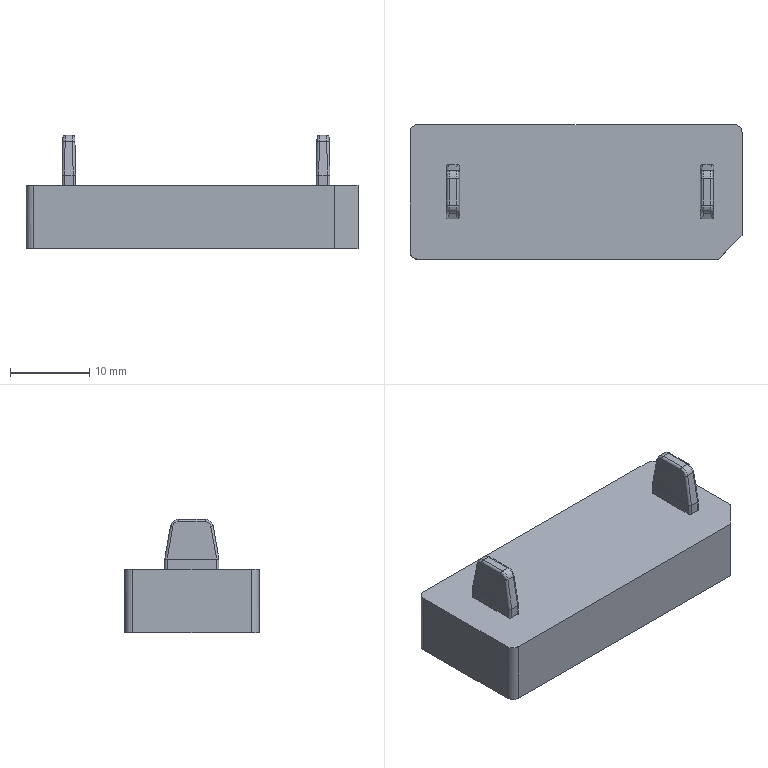NC program | PowerMill | posted by the shop | part box 42 x 17 x 14.346 mm
Lines 3424 to 3987 of 50900:
( TOOL ID   D10_1_1 )
( TOOL DIA. 10. TIP RAD 0 LENGTH 69.52 )
( Z = -.404 )
T3 M6
T4
G91 G28 Z0
G0 G90 G54
M08
S8500 M3
X0 Y0 M8
G43 Z11.796 H3
X-11.962 Y-11.844
Z.796
G1 Z-.404 F360
X-13.457 Y-6.785 F600
X-13.817 Y6.954
X-14.302 Y7.052
X-14.75 Y7.102
X-15.198 Y7.112
X-15.645 Y7.094
X-16.092 Y7.096
X-16.54 Y7.07
X-16.988 Y7.01
X-17.435 Y6.905
X-17.707 Y6.821
X-17.347 Y-6.889
G0 Z3.996
G1 X20.165 Y-11.853 F10000
G0 Z.796
G1 Z-.404 F360
X18.675 Y-6.793 F600
X18.364 Y6.949
X17.881 Y7.048
X17.433 Y7.101
X16.985 Y7.112
X16.538 Y7.091
X16.091 Y7.096
X15.643 Y7.073
X15.195 Y7.015
X14.748 Y6.914
X14.478 Y6.832
X14.788 Y-6.884
G0 Z11.796
X0 Y0
Z9.796
X31.535 Y3.509
Z-5.35
G1 Z-6.55 F360
X26.26 F600
X22.67 Y3.361
X22.675 Y-3.109
X22.665 Y-3.417
X22.639 Y-3.723
X22.59 Y-4.077
X22.516 Y-4.426
X22.42 Y-4.769
G2 X20.666 Y-7.385 I-5.297 J1.655
X19.816 Y-7.966 I-3.572 J4.314
G1 X19.515 Y-8.122
X19.205 Y-8.259
X18.887 Y-8.375
G2 X18.117 Y-8.574 I-1.905 J5.767
G1 X17.764 Y-8.625
X17.409 Y-8.657
X16.722 Y-8.666
X15.751 Y-8.657
X15.396 Y-8.625
X15.043 Y-8.574
X14.685 Y-8.497
X14.273 Y-8.375
G2 X13.295 Y-7.939 I1.765 J5.269
G1 X13.017 Y-7.771
X12.749 Y-7.586
X12.494 Y-7.385
G2 X10.74 Y-4.769 I3.544 J4.271
G1 X10.644 Y-4.426
X10.561 Y-4.008
X10.518 Y-3.698
X10.492 Y-3.385
X10.485 Y-3.109
Y3.148
G2 X10.644 Y4.465 I5.803 J-.031
X10.87 Y5.181 I6.382 J-1.628
G1 X11.001 Y5.486
G2 X11.518 Y6.376 I5.36 J-2.52
G1 X11.749 Y6.675
G2 X13.344 Y8.005 I4.289 J-3.522
G1 X13.645 Y8.161
G2 X14.579 Y8.505 I2.378 J-5.018
X16.036 Y8.704 I1.477 J-5.401
G1 X16.722 Y8.705
X17.409 Y8.696
X17.706 Y8.671
G2 X19.909 Y7.951 I-.58 J-5.501
G1 X20.143 Y7.81
G2 X21.193 Y6.928 I-3.119 J-4.776
G1 X21.425 Y6.658
X21.642 Y6.376
G2 X22.01 Y5.782 I-4.881 J-3.437
G1 X22.159 Y5.486
X22.29 Y5.181
X22.412 Y4.831
G2 X22.67 Y3.361 I-5.38 J-1.702
G1 X26.26 Y3.509
G0 Z2.856
G1 X-31.535 Y.02 F10000
G0 Z-5.35
G1 Z-6.55 F360
X-26.26 F600
X-21.675
Y3.148
X-21.665 Y3.456
X-21.639 Y3.763
X-21.59 Y4.116
X-21.516 Y4.465
G2 X-21.29 Y5.181 I6.452 J-1.651
G1 X-21.162 Y5.481
G2 X-20.821 Y6.109 I5.763 J-2.719
X-20.411 Y6.675 I4.853 J-3.078
G1 X-20.193 Y6.928
G2 X-19.666 Y7.424 I4.215 J-3.942
G1 X-19.411 Y7.625
G2 X-16.179 Y8.702 I3.295 J-4.5
G1 X-15.036 Y8.704
X-14.72 Y8.694
X-14.406 Y8.666
X-14.043 Y8.614
X-13.869 Y8.576
G2 X-13.216 Y8.393 I-1.014 J-4.88
G1 X-12.955 Y8.298
X-12.645 Y8.161
X-12.295 Y7.978
X-12.017 Y7.81
X-11.749 Y7.625
X-11.494 Y7.424
G2 X-10.967 Y6.928 I-3.716 J-4.467
G1 X-10.735 Y6.658
X-10.518 Y6.376
G2 X-9.74 Y4.808 I-4.556 J-3.237
G1 X-9.644 Y4.465
G2 X-9.485 Y3.148 I-5.657 J-1.349
G1 Y.174
X.298 Y.21
X.308 Y-3.307
X.291 Y-3.81
G3 X.454 Y-3.98 I.163 J-.006
G1 X.563
G3 X.725 Y-3.807 I0 J.162
G1 X.461 Y.023
G2 X.507 Y3.684 I22.513 J1.548
G1 X.522 Y3.837
G3 X.406 Y3.97 I-.12 J.011
X.28 Y3.847 I-.005 J-.121
G1 X.298 Y.21
X-4.676 Y.192
X-4.688 Y3.403
G3 X-4.911 Y5.299 I-10.314 J-.251
G1 X-4.952 Y5.491
X-5.182 Y6.32
X-5.415 Y6.967
X-5.79 Y7.862
G2 X-5.067 Y8.955 I.724 J.307
G1 X6.068
G2 X6.791 Y7.863 I0 J-.785
G1 X6.51 Y7.203
G3 X5.413 Y.753 I13.041 J-5.537
G1 X5.714 Y-3.871
G3 X6.094 Y-5.986 I10.404 J.779
G1 X6.227 Y-6.412
X6.369 Y-6.809
X6.527 Y-7.201
X6.811 Y-7.863
G2 X6.092 Y-8.954 I-.719 J-.309
G1 X-5.092 Y-8.955
G2 X-5.803 Y-7.843 I0 J.783
G1 X-5.675 Y-7.566
G3 X-5.169 Y-6.25 I-9.851 J4.544
G1 X-5.141 Y-6.161
G3 X-4.664 Y-2.995 I-10.056 J3.133
G1 X-4.676 Y.192
X-9.485 Y.174
Y-3.109
X-9.495 Y-3.417
X-9.521 Y-3.723
X-9.57 Y-4.077
X-9.644 Y-4.426
G2 X-9.87 Y-5.142 I-6.444 J1.648
X-10.518 Y-6.337 I-5.326 J2.114
X-11.202 Y-7.126 I-4.806 J3.47
X-12.017 Y-7.771 I-4.034 J4.265
X-12.955 Y-8.259 I-3.189 J4.984
X-14.043 Y-8.574 I-2.202 J5.557
G1 X-14.396 Y-8.625
X-14.751 Y-8.657
X-15.036 Y-8.664
X-16.409 Y-8.657
G2 X-17.247 Y-8.546 I.3 J5.522
G1 X-17.475 Y-8.497
X-17.887 Y-8.375
X-18.205 Y-8.259
X-18.515 Y-8.122
X-18.816 Y-7.966
G2 X-21.01 Y-5.743 I2.691 J4.85
X-21.42 Y-4.769 I4.921 J2.643
G1 X-21.516 Y-4.426
X-21.59 Y-4.077
X-21.639 Y-3.723
X-21.665 Y-3.417
X-21.675 Y-3.109
Y.02
X-26.26
G0 Z9.796
X0 Y0
X26.008 Y-14.747
Z-13.25
G1 Z-14.45 F360
G3 X22.473 Y-11.211 I-1.768 J1.768 F600
G1 X21.559 Y-12.125
X21.557 Y-12.127
X21.554 Y-12.129
X21.061 Y-12.554
X21.057 Y-12.557
X21.053 Y-12.56
X20.606 Y-12.861
X20.603 Y-12.862
X20.6 Y-12.864
X20.294 Y-13.033
X20.292 Y-13.034
X20.29 Y-13.035
X20.149 Y-13.103
X20.147 Y-13.104
X20.145 Y-13.105
X19.698 Y-13.288
X19.694 Y-13.289
X19.69 Y-13.29
X19.244 Y-13.425
X19.241 Y-13.426
X19.238 Y-13.427
X18.964 Y-13.488
X18.962
X18.96
X18.787 Y-13.519
X18.785
X18.782
X18.335 Y-13.569
X18.332
X18.328
X17.881 Y-13.58
X17.88
X17.879
X-19.22
X-19.221
X-20.114 Y-13.579
X-20.117
X-20.119
X-20.566 Y-13.552
X-20.569
X-20.572 Y-13.551
X-21.019 Y-13.494
X-21.022 Y-13.493
X-21.025
X-21.472 Y-13.398
X-21.475 Y-13.397
X-21.478 Y-13.396
X-21.925 Y-13.267
X-21.928 Y-13.266
X-21.931 Y-13.265
X-22.378 Y-13.096
X-22.381 Y-13.095
X-22.384 Y-13.093
X-22.831 Y-12.88
X-22.834 Y-12.879
X-22.837 Y-12.877
X-23.284 Y-12.617
X-23.287 Y-12.615
X-23.29 Y-12.613
X-23.737 Y-12.295
X-23.74 Y-12.293
X-23.742 Y-12.29
X-24.189 Y-11.906
X-24.192 Y-11.904
X-24.194 Y-11.901
X-24.416 Y-11.678
X-24.418 Y-11.676
X-24.42 Y-11.674
X-24.803 Y-11.227
X-24.805 Y-11.224
X-24.807 Y-11.221
X-25.096 Y-10.815
X-25.098 Y-10.812
X-25.1 Y-10.809
X-25.385 Y-10.321
X-25.387 Y-10.318
X-25.389 Y-10.315
X-25.6 Y-9.868
X-25.601 Y-9.865
X-25.602 Y-9.862
X-25.77 Y-9.415
X-25.771 Y-9.412
X-25.772 Y-9.409
X-25.9 Y-8.962
X-25.901 Y-8.959
X-25.902 Y-8.956
X-25.995 Y-8.509
X-25.996 Y-8.506
Y-8.503
X-26.053 Y-8.056
Y-8.053
Y-8.05
X-26.079 Y-7.603
Y-7.601
Y-7.599
Y7.599
Y7.601
Y7.603
X-26.053 Y8.05
Y8.053
Y8.055
X-26.005 Y8.454
X-26.004 Y8.457
Y8.46
X-25.902 Y8.956
X-25.901 Y8.959
X-25.9 Y8.962
X-25.772 Y9.409
X-25.771 Y9.412
X-25.77 Y9.415
X-25.602 Y9.862
X-25.601 Y9.865
X-25.6 Y9.868
X-25.389 Y10.315
X-25.387 Y10.318
X-25.386 Y10.321
X-25.127 Y10.768
X-25.125 Y10.771
X-25.123 Y10.774
X-24.807 Y11.221
X-24.805 Y11.224
X-24.803 Y11.227
X-24.42 Y11.674
X-24.418 Y11.676
X-24.416 Y11.678
X-24.194 Y11.901
X-24.192 Y11.904
X-24.189 Y11.906
X-23.742 Y12.29
X-23.74 Y12.292
X-23.737 Y12.295
X-23.34 Y12.581
X-23.337 Y12.583
X-23.334 Y12.585
X-22.837 Y12.877
X-22.834 Y12.879
X-22.831 Y12.88
X-22.384 Y13.093
X-22.381 Y13.095
X-22.378 Y13.096
X-21.931 Y13.265
X-21.928 Y13.266
X-21.925 Y13.267
X-21.478 Y13.396
X-21.475 Y13.397
X-21.472 Y13.398
X-21.053 Y13.488
X-21.05
X-21.046 Y13.489
X-20.572 Y13.551
X-20.569 Y13.552
X-20.566
X-20.119 Y13.579
X-20.117
X-20.115
X-19.668 Y13.58
X-19.667
X-.223
X19.22
X19.221
X20.114 Y13.579
X20.117
X20.119
X20.566 Y13.552
X20.569
X20.572 Y13.551
X21.019 Y13.494
X21.022 Y13.493
X21.025
X21.472 Y13.398
X21.475 Y13.397
X21.478 Y13.396
X21.925 Y13.267
X21.928 Y13.266
X21.931 Y13.265
X22.378 Y13.096
X22.381 Y13.094
X22.384 Y13.093
X22.831 Y12.88
X22.834 Y12.879
X22.837 Y12.877
X23.284 Y12.617
X23.287 Y12.615
X23.29 Y12.613
X23.737 Y12.295
X23.74 Y12.293
X23.742 Y12.29
X24.189 Y11.906
X24.192 Y11.904
X24.194 Y11.901
X24.416 Y11.678
X24.418 Y11.676
X24.42 Y11.674
X24.803 Y11.227
X24.805 Y11.224
X24.807 Y11.221
X25.096 Y10.815
X25.098 Y10.812
X25.1 Y10.809
X25.385 Y10.321
X25.387 Y10.318
X25.389 Y10.315
X25.6 Y9.868
X25.601 Y9.865
X25.602 Y9.862
X25.77 Y9.415
X25.771 Y9.412
X25.772 Y9.409
X25.9 Y8.962
X25.901 Y8.959
X25.902 Y8.956
X25.995 Y8.509
X25.996 Y8.506
Y8.503
X26.053 Y8.056
Y8.053
Y8.05
X26.079 Y7.603
Y7.601
Y7.599
X26.08 Y-5.364
Y-5.365
Y-5.366
X26.07 Y-5.813
Y-5.816
Y-5.819
X26.022 Y-6.266
X26.021 Y-6.27
Y-6.274
X25.931 Y-6.72
X25.93 Y-6.724
X25.929 Y-6.728
X25.796 Y-7.175
X25.795 Y-7.178
X25.793 Y-7.182
X25.612 Y-7.629
X25.611 Y-7.631
X25.61 Y-7.633
X25.55 Y-7.759
X25.549 Y-7.76
X25.548 Y-7.762
X25.374 Y-8.084
X25.372 Y-8.087
X25.37 Y-8.09
X25.098 Y-8.502
X25.095 Y-8.506
X25.092 Y-8.51
X24.645 Y-9.038
X24.643 Y-9.04
X24.641 Y-9.043
X22.473 Y-11.211
G3 X26.008 Y-14.747 I1.768 J-1.768
G1 X25.957 Y-14.685
G3 X22.421 Y-11.149 I-1.768 J1.768
G1 X21.502 Y-12.069
X21.008 Y-12.494
X20.561 Y-12.794
X20.255 Y-12.963
X20.114 Y-13.031
X19.667 Y-13.214
X19.22 Y-13.349
X18.947 Y-13.41
X18.773 Y-13.44
X18.326 Y-13.489
X17.879 Y-13.5
X-19.22
X-20.114 Y-13.499
X-20.561 Y-13.472
X-21.008 Y-13.414
X-21.455 Y-13.319
X-21.902 Y-13.19
X-22.349 Y-13.021
X-22.796 Y-12.808
X-23.243 Y-12.548
X-23.69 Y-12.23
X-24.137 Y-11.845
X-24.36 Y-11.622
X-24.742 Y-11.175
X-25.031 Y-10.769
X-25.316 Y-10.281
X-25.528 Y-9.834
X-25.695 Y-9.387
X-25.823 Y-8.94
X-25.917 Y-8.493
X-25.973 Y-8.046
X-25.999 Y-7.599
Y7.599
X-25.973 Y8.046
X-25.925 Y8.444
X-25.823 Y8.94
X-25.695 Y9.387
X-25.528 Y9.834
X-25.316 Y10.281
X-25.058 Y10.728
X-24.742 Y11.175
X-24.36 Y11.622
X-24.137 Y11.845
X-23.69 Y12.23
X-23.293 Y12.516
X-22.796 Y12.808
X-22.349 Y13.021
X-21.902 Y13.19
X-21.455 Y13.319
X-21.036 Y13.41
X-20.561 Y13.472
X-20.114 Y13.499
X-19.667 Y13.5
X-.223
X19.22
X20.114 Y13.499
X20.561 Y13.472
X21.008 Y13.414
X21.455 Y13.319
X21.902 Y13.19
X22.349 Y13.021
X22.796 Y12.808
X23.243 Y12.548
X23.69 Y12.23
X24.137 Y11.845
X24.36 Y11.622
X24.742 Y11.175
X25.031 Y10.769
X25.316 Y10.281
X25.528 Y9.834
X25.695 Y9.387
X25.823 Y8.94
X25.917 Y8.493
X25.973 Y8.046
X25.999 Y7.599
X26. Y-5.364
X25.99 Y-5.811
X25.942 Y-6.258
X25.853 Y-6.705
X25.719 Y-7.152
X25.538 Y-7.599
X25.478 Y-7.724
X25.303 Y-8.046
X25.031 Y-8.458
X24.584 Y-8.986
X22.421 Y-11.149
G3 X25.957 Y-14.685 I1.768 J-1.768
G0 Z9.796
Z10.796
X0 Y0
M9
M5
M01